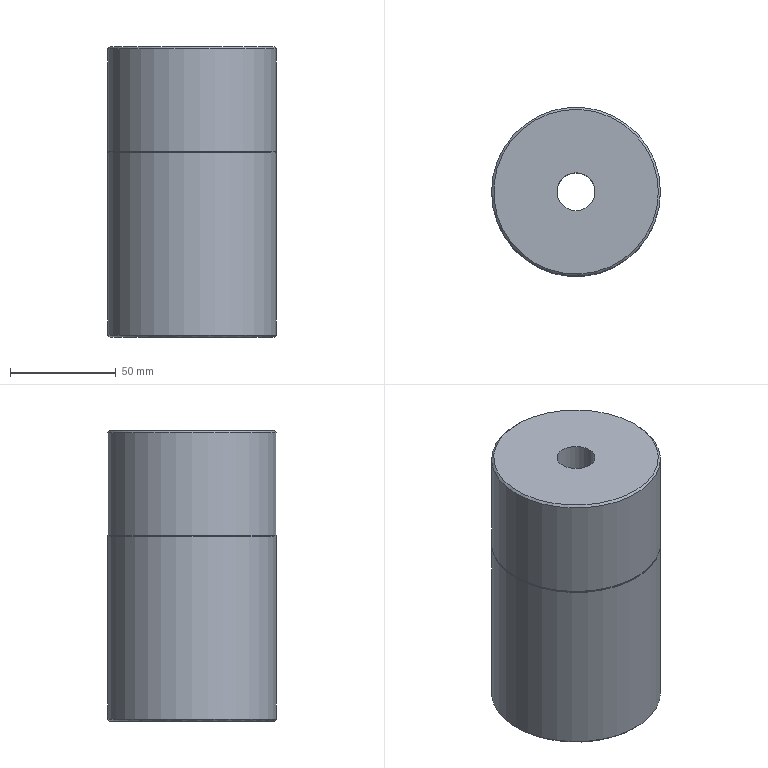Part | STEP file | 014_id2546_x_t | 1 solid | 12 faces | box 80 x 80 x 137.5 mm | volume 639951 mm3 | cylinder 5 | plane 5 | cone 2 | commonest cylinder face diameters 80 x2 18.009 x1 26.008 x1 79.6 x1
STEP:
#1=CARTESIAN_POINT('',(2407.435,555.,93.));
#2=VERTEX_POINT('',#1);
#3=CARTESIAN_POINT('',(2367.435,555.,93.));
#4=DIRECTION('',(0.,0.,1.));
#5=DIRECTION('',(1.,0.,0.));
#6=AXIS2_PLACEMENT_3D('',#3,#4,#5);
#7=CIRCLE('',#6,40.);
#8=EDGE_CURVE('',#2,#2,#7,.T.);
#9=ORIENTED_EDGE('',*,*,#8,.T.);
#10=EDGE_LOOP('',(#9));
#11=FACE_BOUND('',#10,.T.);
#12=CARTESIAN_POINT('',(2407.435,555.,141.5));
#13=VERTEX_POINT('',#12);
#14=CARTESIAN_POINT('',(2367.435,555.,141.5));
#15=DIRECTION('',(0.,0.,-1.));
#16=DIRECTION('',(1.,0.,0.));
#17=AXIS2_PLACEMENT_3D('',#14,#15,#16);
#18=CIRCLE('',#17,40.);
#19=EDGE_CURVE('',#13,#13,#18,.T.);
#20=ORIENTED_EDGE('',*,*,#19,.T.);
#21=EDGE_LOOP('',(#20));
#22=FACE_BOUND('',#21,.T.);
#23=CARTESIAN_POINT('',(2367.435,555.,-66.061));
#24=DIRECTION('',(0.,0.,1.));
#25=DIRECTION('',(1.,0.,0.));
#26=AXIS2_PLACEMENT_3D('',#23,#24,#25);
#27=CYLINDRICAL_SURFACE('',#26,40.);
#28=ADVANCED_FACE('',(#11,#22),#27,.T.);
#29=CARTESIAN_POINT('',(2367.435,541.996,5.));
#30=VERTEX_POINT('',#29);
#31=CARTESIAN_POINT('',(2367.435,555.,5.));
#32=DIRECTION('',(0.,0.,-1.));
#33=DIRECTION('',(0.,-1.,0.));
#34=AXIS2_PLACEMENT_3D('',#31,#32,#33);
#35=CIRCLE('',#34,13.004);
#36=EDGE_CURVE('',#30,#30,#35,.T.);
#37=ORIENTED_EDGE('',*,*,#36,.F.);
#38=EDGE_LOOP('',(#37));
#39=FACE_BOUND('',#38,.T.);
#40=CARTESIAN_POINT('',(2406.435,555.,5.));
#41=VERTEX_POINT('',#40);
#42=CARTESIAN_POINT('',(2367.435,555.,5.));
#43=DIRECTION('',(0.,0.,-1.));
#44=DIRECTION('',(1.,0.,0.));
#45=AXIS2_PLACEMENT_3D('',#42,#43,#44);
#46=CIRCLE('',#45,39.);
#47=EDGE_CURVE('',#41,#41,#46,.T.);
#48=ORIENTED_EDGE('',*,*,#47,.T.);
#49=EDGE_LOOP('',(#48));
#50=FACE_BOUND('',#49,.T.);
#51=CARTESIAN_POINT('',(2367.435,594.,5.));
#52=DIRECTION('',(0.,0.,-1.));
#53=DIRECTION('',(-1.,0.,0.));
#54=AXIS2_PLACEMENT_3D('',#51,#52,#53);
#55=PLANE('',#54);
#56=ADVANCED_FACE('',(#39,#50),#55,.T.);
#57=ORIENTED_EDGE('',*,*,#19,.F.);
#58=EDGE_LOOP('',(#57));
#59=FACE_BOUND('',#58,.T.);
#60=CARTESIAN_POINT('',(2406.435,555.,142.5));
#61=VERTEX_POINT('',#60);
#62=CARTESIAN_POINT('',(2367.435,555.,142.5));
#63=DIRECTION('',(0.,0.,-1.));
#64=DIRECTION('',(1.,0.,0.));
#65=AXIS2_PLACEMENT_3D('',#62,#63,#64);
#66=CIRCLE('',#65,39.);
#67=EDGE_CURVE('',#61,#61,#66,.T.);
#68=ORIENTED_EDGE('',*,*,#67,.T.);
#69=EDGE_LOOP('',(#68));
#70=FACE_BOUND('',#69,.T.);
#71=CARTESIAN_POINT('',(2367.435,555.,142.5));
#72=DIRECTION('',(0.,0.,-1.));
#73=DIRECTION('',(-1.,0.,0.));
#74=AXIS2_PLACEMENT_3D('',#71,#72,#73);
#75=CONICAL_SURFACE('',#74,39.,45.);
#76=ADVANCED_FACE('',(#59,#70),#75,.T.);
#77=CARTESIAN_POINT('',(2407.435,555.,92.5));
#78=VERTEX_POINT('',#77);
#79=CARTESIAN_POINT('',(2367.435,555.,92.5));
#80=DIRECTION('',(0.,0.,-1.));
#81=DIRECTION('',(1.,0.,0.));
#82=AXIS2_PLACEMENT_3D('',#79,#80,#81);
#83=CIRCLE('',#82,40.);
#84=EDGE_CURVE('',#78,#78,#83,.T.);
#85=ORIENTED_EDGE('',*,*,#84,.T.);
#86=EDGE_LOOP('',(#85));
#87=FACE_BOUND('',#86,.T.);
#88=CARTESIAN_POINT('',(2407.435,555.,6.));
#89=VERTEX_POINT('',#88);
#90=CARTESIAN_POINT('',(2367.435,555.,6.));
#91=DIRECTION('',(0.,0.,-1.));
#92=DIRECTION('',(1.,0.,0.));
#93=AXIS2_PLACEMENT_3D('',#90,#91,#92);
#94=CIRCLE('',#93,40.);
#95=EDGE_CURVE('',#89,#89,#94,.T.);
#96=ORIENTED_EDGE('',*,*,#95,.F.);
#97=EDGE_LOOP('',(#96));
#98=FACE_BOUND('',#97,.T.);
#99=CARTESIAN_POINT('',(2367.435,555.,-3.561));
#100=DIRECTION('',(0.,0.,1.));
#101=DIRECTION('',(1.,0.,0.));
#102=AXIS2_PLACEMENT_3D('',#99,#100,#101);
#103=CYLINDRICAL_SURFACE('',#102,40.);
#104=ADVANCED_FACE('',(#87,#98),#103,.T.);
#105=ORIENTED_EDGE('',*,*,#47,.F.);
#106=EDGE_LOOP('',(#105));
#107=FACE_BOUND('',#106,.T.);
#108=ORIENTED_EDGE('',*,*,#95,.T.);
#109=EDGE_LOOP('',(#108));
#110=FACE_BOUND('',#109,.T.);
#111=CARTESIAN_POINT('',(2367.435,555.,6.));
#112=DIRECTION('',(0.,0.,1.));
#113=DIRECTION('',(1.,0.,0.));
#114=AXIS2_PLACEMENT_3D('',#111,#112,#113);
#115=CONICAL_SURFACE('',#114,40.,45.);
#116=ADVANCED_FACE('',(#107,#110),#115,.T.);
#117=CARTESIAN_POINT('',(2367.435,564.004,142.5));
#118=VERTEX_POINT('',#117);
#119=CARTESIAN_POINT('',(2367.435,555.,142.5));
#120=DIRECTION('',(0.,0.,1.));
#121=DIRECTION('',(0.,1.,0.));
#122=AXIS2_PLACEMENT_3D('',#119,#120,#121);
#123=CIRCLE('',#122,9.005);
#124=EDGE_CURVE('',#118,#118,#123,.T.);
#125=ORIENTED_EDGE('',*,*,#124,.F.);
#126=EDGE_LOOP('',(#125));
#127=FACE_BOUND('',#126,.T.);
#128=ORIENTED_EDGE('',*,*,#67,.F.);
#129=EDGE_LOOP('',(#128));
#130=FACE_BOUND('',#129,.T.);
#131=CARTESIAN_POINT('',(2367.435,560.5,142.5));
#132=DIRECTION('',(0.,0.,1.));
#133=DIRECTION('',(1.,0.,0.));
#134=AXIS2_PLACEMENT_3D('',#131,#132,#133);
#135=PLANE('',#134);
#136=ADVANCED_FACE('',(#127,#130),#135,.T.);
#137=ORIENTED_EDGE('',*,*,#8,.F.);
#138=EDGE_LOOP('',(#137));
#139=FACE_BOUND('',#138,.T.);
#140=CARTESIAN_POINT('',(2367.435,515.2,93.));
#141=VERTEX_POINT('',#140);
#142=CARTESIAN_POINT('',(2367.435,555.,93.));
#143=DIRECTION('',(0.,0.,-1.));
#144=DIRECTION('',(0.,-1.,0.));
#145=AXIS2_PLACEMENT_3D('',#142,#143,#144);
#146=CIRCLE('',#145,39.8);
#147=EDGE_CURVE('',#141,#141,#146,.T.);
#148=ORIENTED_EDGE('',*,*,#147,.F.);
#149=EDGE_LOOP('',(#148));
#150=FACE_BOUND('',#149,.T.);
#151=CARTESIAN_POINT('',(2367.435,555.,93.));
#152=DIRECTION('',(0.,0.,1.));
#153=DIRECTION('',(1.,0.,0.));
#154=AXIS2_PLACEMENT_3D('',#151,#152,#153);
#155=PLANE('',#154);
#156=ADVANCED_FACE('',(#139,#150),#155,.F.);
#157=ORIENTED_EDGE('',*,*,#84,.F.);
#158=EDGE_LOOP('',(#157));
#159=FACE_BOUND('',#158,.T.);
#160=CARTESIAN_POINT('',(2367.435,515.2,92.5));
#161=VERTEX_POINT('',#160);
#162=CARTESIAN_POINT('',(2367.435,555.,92.5));
#163=DIRECTION('',(0.,0.,-1.));
#164=DIRECTION('',(0.,-1.,0.));
#165=AXIS2_PLACEMENT_3D('',#162,#163,#164);
#166=CIRCLE('',#165,39.8);
#167=EDGE_CURVE('',#161,#161,#166,.T.);
#168=ORIENTED_EDGE('',*,*,#167,.T.);
#169=EDGE_LOOP('',(#168));
#170=FACE_BOUND('',#169,.T.);
#171=CARTESIAN_POINT('',(2367.435,555.,92.5));
#172=DIRECTION('',(0.,0.,1.));
#173=DIRECTION('',(1.,0.,0.));
#174=AXIS2_PLACEMENT_3D('',#171,#172,#173);
#175=PLANE('',#174);
#176=ADVANCED_FACE('',(#159,#170),#175,.T.);
#177=ORIENTED_EDGE('',*,*,#147,.T.);
#178=EDGE_LOOP('',(#177));
#179=FACE_BOUND('',#178,.T.);
#180=ORIENTED_EDGE('',*,*,#167,.F.);
#181=EDGE_LOOP('',(#180));
#182=FACE_BOUND('',#181,.T.);
#183=CARTESIAN_POINT('',(2367.435,555.,93.));
#184=DIRECTION('',(0.,0.,-1.));
#185=DIRECTION('',(0.,-1.,0.));
#186=AXIS2_PLACEMENT_3D('',#183,#184,#185);
#187=CYLINDRICAL_SURFACE('',#186,39.8);
#188=ADVANCED_FACE('',(#179,#182),#187,.T.);
#189=ORIENTED_EDGE('',*,*,#124,.T.);
#190=EDGE_LOOP('',(#189));
#191=FACE_BOUND('',#190,.T.);
#192=CARTESIAN_POINT('',(2367.435,564.004,62.5));
#193=VERTEX_POINT('',#192);
#194=CARTESIAN_POINT('',(2367.435,555.,62.5));
#195=DIRECTION('',(0.,0.,1.));
#196=DIRECTION('',(0.,1.,0.));
#197=AXIS2_PLACEMENT_3D('',#194,#195,#196);
#198=CIRCLE('',#197,9.005);
#199=EDGE_CURVE('',#193,#193,#198,.T.);
#200=ORIENTED_EDGE('',*,*,#199,.F.);
#201=EDGE_LOOP('',(#200));
#202=FACE_BOUND('',#201,.T.);
#203=CARTESIAN_POINT('',(2367.435,555.,43.5));
#204=DIRECTION('',(0.,0.,1.));
#205=DIRECTION('',(-1.,0.,0.));
#206=AXIS2_PLACEMENT_3D('',#203,#204,#205);
#207=CYLINDRICAL_SURFACE('',#206,9.005);
#208=ADVANCED_FACE('',(#191,#202),#207,.F.);
#209=ORIENTED_EDGE('',*,*,#199,.T.);
#210=EDGE_LOOP('',(#209));
#211=FACE_BOUND('',#210,.T.);
#212=CARTESIAN_POINT('',(2354.431,555.,62.5));
#213=VERTEX_POINT('',#212);
#214=CARTESIAN_POINT('',(2367.435,555.,62.5));
#215=DIRECTION('',(0.,0.,1.));
#216=DIRECTION('',(-1.,0.,0.));
#217=AXIS2_PLACEMENT_3D('',#214,#215,#216);
#218=CIRCLE('',#217,13.004);
#219=EDGE_CURVE('',#213,#213,#218,.T.);
#220=ORIENTED_EDGE('',*,*,#219,.F.);
#221=EDGE_LOOP('',(#220));
#222=FACE_BOUND('',#221,.T.);
#223=CARTESIAN_POINT('',(2367.435,555.,62.5));
#224=DIRECTION('',(0.,0.,1.));
#225=DIRECTION('',(0.,1.,0.));
#226=AXIS2_PLACEMENT_3D('',#223,#224,#225);
#227=PLANE('',#226);
#228=ADVANCED_FACE('',(#211,#222),#227,.F.);
#229=ORIENTED_EDGE('',*,*,#36,.T.);
#230=EDGE_LOOP('',(#229));
#231=FACE_BOUND('',#230,.T.);
#232=ORIENTED_EDGE('',*,*,#219,.T.);
#233=EDGE_LOOP('',(#232));
#234=FACE_BOUND('',#233,.T.);
#235=CARTESIAN_POINT('',(2367.435,555.,43.5));
#236=DIRECTION('',(0.,0.,1.));
#237=DIRECTION('',(-1.,0.,0.));
#238=AXIS2_PLACEMENT_3D('',#235,#236,#237);
#239=CYLINDRICAL_SURFACE('',#238,13.004);
#240=ADVANCED_FACE('',(#231,#234),#239,.F.);
#241=CLOSED_SHELL('',(#28,#56,#76,#104,#116,#136,#156,#176,#188,#208,#228,#240));
#242=MANIFOLD_SOLID_BREP('',#241);
#243=(LENGTH_UNIT()NAMED_UNIT(*)SI_UNIT(.MILLI.,.METRE.));
#244=UNCERTAINTY_MEASURE_WITH_UNIT(LENGTH_MEASURE(0.00002),#243,'','');
#245=(NAMED_UNIT(*)PLANE_ANGLE_UNIT()SI_UNIT($,.RADIAN.));
#246=PLANE_ANGLE_MEASURE_WITH_UNIT(PLANE_ANGLE_MEASURE(0.01745),#245);
#247=DIMENSIONAL_EXPONENTS(0.,0.,0.,0.,0.,0.,0.);
#248=(CONVERSION_BASED_UNIT('DEGREE',#246)NAMED_UNIT(#247)PLANE_ANGLE_UNIT());
#249=(NAMED_UNIT(*)SI_UNIT($,.STERADIAN.)SOLID_ANGLE_UNIT());
#250=(GEOMETRIC_REPRESENTATION_CONTEXT(3)GLOBAL_UNCERTAINTY_ASSIGNED_CONTEXT((#244))GLOBAL_UNIT_ASSIGNED_CONTEXT((#243,#248,#249))REPRESENTATION_CONTEXT('',''));
#251=ADVANCED_BREP_SHAPE_REPRESENTATION('',(#242),#250);